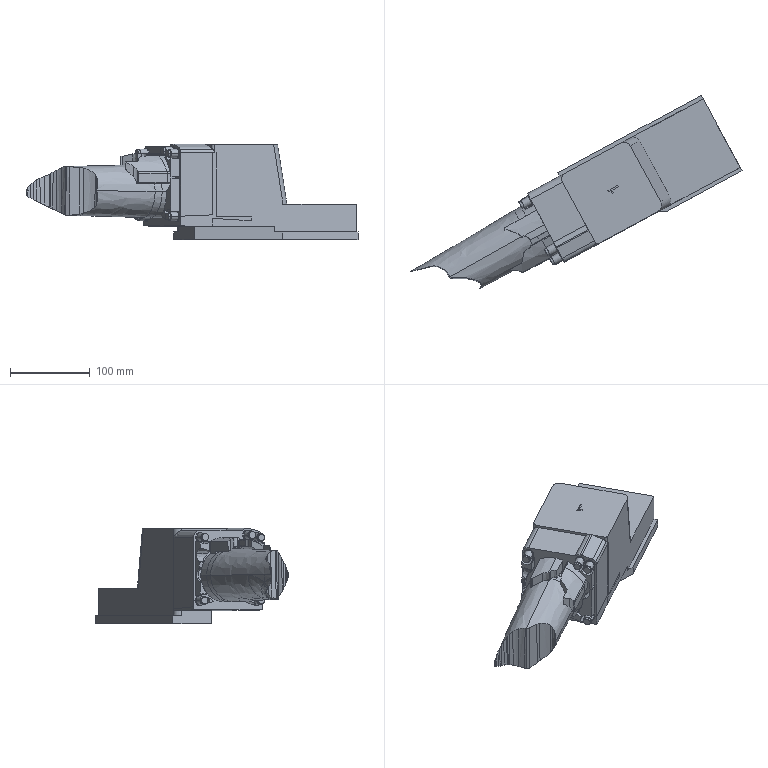Part | Creo | 1 solid | 235 faces | box 417.131 x 242.941 x 120.324 mm | volume 2559820 mm3 | plane 86 | cylinder 68 | cone 38 | spline 37 | other 6 | commonest cylinder face diameters 8.643 x10 10.653 x10 12.663 x10 14.768 x2 18 x2 78.935 x2